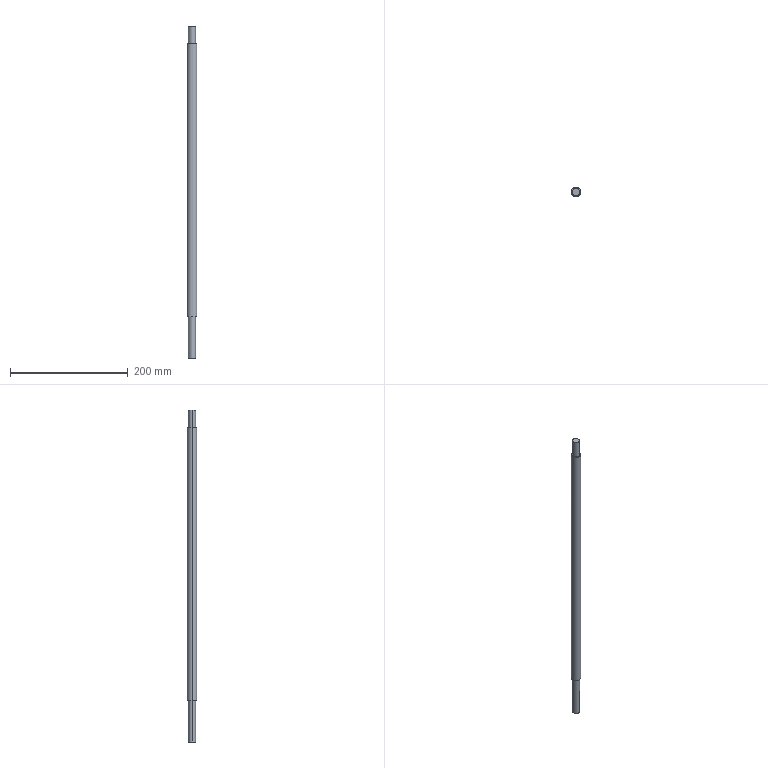Part | SolidWorks | features ICE 2, Extrusion 1 | 1 solid | 10 faces | box 16 x 16 x 563.4 mm | volume 104482 mm3 | cylinder 6 | plane 4 | commonest cylinder face diameters 12 x4 16 x2
STEP:
#1=CARTESIAN_POINT('',(-6.,0.,-301.7));
#2=VERTEX_POINT('',#1);
#3=CARTESIAN_POINT('',(6.,0.,-301.7));
#4=VERTEX_POINT('',#3);
#5=CARTESIAN_POINT('',(0.,0.,-301.7));
#6=DIRECTION('',(0.,0.,-1.));
#7=DIRECTION('',(-1.,0.,0.));
#8=AXIS2_PLACEMENT_3D('',#5,#6,#7);
#9=CIRCLE('',#8,6.);
#10=EDGE_CURVE('',#2,#4,#9,.T.);
#11=ORIENTED_EDGE('',*,*,#10,.F.);
#12=CARTESIAN_POINT('',(-6.,0.,-231.7));
#13=VERTEX_POINT('',#12);
#14=CARTESIAN_POINT('',(-6.,0.,-301.7));
#15=DIRECTION('',(0.,0.,1.));
#16=VECTOR('',#15,1000.);
#17=LINE('',#14,#16);
#18=EDGE_CURVE('',#2,#13,#17,.T.);
#19=ORIENTED_EDGE('',*,*,#18,.T.);
#20=CARTESIAN_POINT('',(6.,0.,-231.7));
#21=VERTEX_POINT('',#20);
#22=CARTESIAN_POINT('',(0.,0.,-231.7));
#23=DIRECTION('',(0.,0.,-1.));
#24=DIRECTION('',(1.,0.,0.));
#25=AXIS2_PLACEMENT_3D('',#22,#23,#24);
#26=CIRCLE('',#25,6.);
#27=EDGE_CURVE('',#13,#21,#26,.T.);
#28=ORIENTED_EDGE('',*,*,#27,.T.);
#29=CARTESIAN_POINT('',(6.,0.,-301.7));
#30=DIRECTION('',(0.,0.,1.));
#31=VECTOR('',#30,1000.);
#32=LINE('',#29,#31);
#33=EDGE_CURVE('',#4,#21,#32,.T.);
#34=ORIENTED_EDGE('',*,*,#33,.F.);
#35=EDGE_LOOP('',(#11,#19,#28,#34));
#36=FACE_OUTER_BOUND('',#35,.T.);
#37=CARTESIAN_POINT('',(0.,0.,-301.7));
#38=DIRECTION('',(0.,0.,1.));
#39=DIRECTION('',(1.,0.,0.));
#40=AXIS2_PLACEMENT_3D('',#37,#38,#39);
#41=CYLINDRICAL_SURFACE('',#40,6.);
#42=ADVANCED_FACE('',(#36),#41,.T.);
#43=CARTESIAN_POINT('',(6.,0.,261.7));
#44=VERTEX_POINT('',#43);
#45=CARTESIAN_POINT('',(-6.,0.,261.7));
#46=VERTEX_POINT('',#45);
#47=CARTESIAN_POINT('',(0.,0.,261.7));
#48=DIRECTION('',(0.,0.,1.));
#49=DIRECTION('',(1.,0.,0.));
#50=AXIS2_PLACEMENT_3D('',#47,#48,#49);
#51=CIRCLE('',#50,6.);
#52=EDGE_CURVE('',#44,#46,#51,.T.);
#53=ORIENTED_EDGE('',*,*,#52,.F.);
#54=CARTESIAN_POINT('',(6.,0.,231.7));
#55=VERTEX_POINT('',#54);
#56=CARTESIAN_POINT('',(6.,0.,261.7));
#57=DIRECTION('',(0.,0.,-1.));
#58=VECTOR('',#57,1000.);
#59=LINE('',#56,#58);
#60=EDGE_CURVE('',#44,#55,#59,.T.);
#61=ORIENTED_EDGE('',*,*,#60,.T.);
#62=CARTESIAN_POINT('',(-6.,0.,231.7));
#63=VERTEX_POINT('',#62);
#64=CARTESIAN_POINT('',(0.,0.,231.7));
#65=DIRECTION('',(0.,0.,1.));
#66=DIRECTION('',(1.,0.,0.));
#67=AXIS2_PLACEMENT_3D('',#64,#65,#66);
#68=CIRCLE('',#67,6.);
#69=EDGE_CURVE('',#55,#63,#68,.T.);
#70=ORIENTED_EDGE('',*,*,#69,.T.);
#71=CARTESIAN_POINT('',(-6.,0.,261.7));
#72=DIRECTION('',(0.,0.,-1.));
#73=VECTOR('',#72,1000.);
#74=LINE('',#71,#73);
#75=EDGE_CURVE('',#46,#63,#74,.T.);
#76=ORIENTED_EDGE('',*,*,#75,.F.);
#77=EDGE_LOOP('',(#53,#61,#70,#76));
#78=FACE_OUTER_BOUND('',#77,.T.);
#79=CARTESIAN_POINT('',(0.,0.,261.7));
#80=DIRECTION('',(0.,0.,-1.));
#81=DIRECTION('',(-1.,0.,0.));
#82=AXIS2_PLACEMENT_3D('',#79,#80,#81);
#83=CYLINDRICAL_SURFACE('',#82,6.);
#84=ADVANCED_FACE('',(#78),#83,.T.);
#85=CARTESIAN_POINT('',(8.,0.,231.7));
#86=VERTEX_POINT('',#85);
#87=CARTESIAN_POINT('',(-8.,0.,231.7));
#88=VERTEX_POINT('',#87);
#89=CARTESIAN_POINT('',(0.,0.,231.7));
#90=DIRECTION('',(0.,0.,1.));
#91=DIRECTION('',(1.,0.,0.));
#92=AXIS2_PLACEMENT_3D('',#89,#90,#91);
#93=CIRCLE('',#92,8.);
#94=EDGE_CURVE('',#86,#88,#93,.T.);
#95=ORIENTED_EDGE('',*,*,#94,.F.);
#96=CARTESIAN_POINT('',(8.,0.,-231.7));
#97=VERTEX_POINT('',#96);
#98=CARTESIAN_POINT('',(8.,0.,231.7));
#99=DIRECTION('',(0.,0.,-1.));
#100=VECTOR('',#99,1000.);
#101=LINE('',#98,#100);
#102=EDGE_CURVE('',#86,#97,#101,.T.);
#103=ORIENTED_EDGE('',*,*,#102,.T.);
#104=CARTESIAN_POINT('',(-8.,0.,-231.7));
#105=VERTEX_POINT('',#104);
#106=CARTESIAN_POINT('',(0.,0.,-231.7));
#107=DIRECTION('',(0.,0.,1.));
#108=DIRECTION('',(1.,0.,0.));
#109=AXIS2_PLACEMENT_3D('',#106,#107,#108);
#110=CIRCLE('',#109,8.);
#111=EDGE_CURVE('',#97,#105,#110,.T.);
#112=ORIENTED_EDGE('',*,*,#111,.T.);
#113=CARTESIAN_POINT('',(-8.,0.,231.7));
#114=DIRECTION('',(0.,0.,-1.));
#115=VECTOR('',#114,1000.);
#116=LINE('',#113,#115);
#117=EDGE_CURVE('',#88,#105,#116,.T.);
#118=ORIENTED_EDGE('',*,*,#117,.F.);
#119=EDGE_LOOP('',(#95,#103,#112,#118));
#120=FACE_OUTER_BOUND('',#119,.T.);
#121=CARTESIAN_POINT('',(0.,0.,231.7));
#122=DIRECTION('',(0.,0.,-1.));
#123=DIRECTION('',(-1.,0.,0.));
#124=AXIS2_PLACEMENT_3D('',#121,#122,#123);
#125=CYLINDRICAL_SURFACE('',#124,8.);
#126=ADVANCED_FACE('',(#120),#125,.T.);
#127=CARTESIAN_POINT('',(0.,0.,-231.7));
#128=DIRECTION('',(0.,0.,1.));
#129=DIRECTION('',(1.,0.,0.));
#130=AXIS2_PLACEMENT_3D('',#127,#128,#129);
#131=CIRCLE('',#130,8.);
#132=EDGE_CURVE('',#105,#97,#131,.T.);
#133=ORIENTED_EDGE('',*,*,#132,.F.);
#134=ORIENTED_EDGE('',*,*,#111,.F.);
#135=EDGE_LOOP('',(#133,#134));
#136=FACE_OUTER_BOUND('',#135,.T.);
#137=CARTESIAN_POINT('',(0.,0.,-231.7));
#138=DIRECTION('',(0.,0.,-1.));
#139=DIRECTION('',(1.,0.,0.));
#140=AXIS2_PLACEMENT_3D('',#137,#138,#139);
#141=CIRCLE('',#140,6.);
#142=EDGE_CURVE('',#21,#13,#141,.T.);
#143=ORIENTED_EDGE('',*,*,#142,.F.);
#144=ORIENTED_EDGE('',*,*,#27,.F.);
#145=EDGE_LOOP('',(#143,#144));
#146=FACE_BOUND('',#145,.T.);
#147=CARTESIAN_POINT('',(0.,0.,-231.7));
#148=DIRECTION('',(0.,0.,1.));
#149=DIRECTION('',(1.,0.,0.));
#150=AXIS2_PLACEMENT_3D('',#147,#148,#149);
#151=PLANE('',#150);
#152=ADVANCED_FACE('',(#136,#146),#151,.F.);
#153=CARTESIAN_POINT('',(0.,0.,231.7));
#154=DIRECTION('',(0.,0.,1.));
#155=DIRECTION('',(1.,0.,0.));
#156=AXIS2_PLACEMENT_3D('',#153,#154,#155);
#157=CIRCLE('',#156,8.);
#158=EDGE_CURVE('',#88,#86,#157,.T.);
#159=ORIENTED_EDGE('',*,*,#158,.T.);
#160=ORIENTED_EDGE('',*,*,#94,.T.);
#161=EDGE_LOOP('',(#159,#160));
#162=FACE_OUTER_BOUND('',#161,.T.);
#163=CARTESIAN_POINT('',(0.,0.,231.7));
#164=DIRECTION('',(0.,0.,1.));
#165=DIRECTION('',(1.,0.,0.));
#166=AXIS2_PLACEMENT_3D('',#163,#164,#165);
#167=CIRCLE('',#166,6.);
#168=EDGE_CURVE('',#63,#55,#167,.T.);
#169=ORIENTED_EDGE('',*,*,#168,.F.);
#170=ORIENTED_EDGE('',*,*,#69,.F.);
#171=EDGE_LOOP('',(#169,#170));
#172=FACE_BOUND('',#171,.T.);
#173=CARTESIAN_POINT('',(0.,0.,231.7));
#174=DIRECTION('',(0.,0.,1.));
#175=DIRECTION('',(1.,0.,0.));
#176=AXIS2_PLACEMENT_3D('',#173,#174,#175);
#177=PLANE('',#176);
#178=ADVANCED_FACE('',(#162,#172),#177,.T.);
#179=ORIENTED_EDGE('',*,*,#102,.F.);
#180=ORIENTED_EDGE('',*,*,#158,.F.);
#181=ORIENTED_EDGE('',*,*,#117,.T.);
#182=ORIENTED_EDGE('',*,*,#132,.T.);
#183=EDGE_LOOP('',(#179,#180,#181,#182));
#184=FACE_OUTER_BOUND('',#183,.T.);
#185=CARTESIAN_POINT('',(0.,0.,231.7));
#186=DIRECTION('',(0.,0.,-1.));
#187=DIRECTION('',(-1.,0.,0.));
#188=AXIS2_PLACEMENT_3D('',#185,#186,#187);
#189=CYLINDRICAL_SURFACE('',#188,8.);
#190=ADVANCED_FACE('',(#184),#189,.T.);
#191=ORIENTED_EDGE('',*,*,#60,.F.);
#192=CARTESIAN_POINT('',(0.,0.,261.7));
#193=DIRECTION('',(0.,0.,1.));
#194=DIRECTION('',(1.,0.,0.));
#195=AXIS2_PLACEMENT_3D('',#192,#193,#194);
#196=CIRCLE('',#195,6.);
#197=EDGE_CURVE('',#46,#44,#196,.T.);
#198=ORIENTED_EDGE('',*,*,#197,.F.);
#199=ORIENTED_EDGE('',*,*,#75,.T.);
#200=ORIENTED_EDGE('',*,*,#168,.T.);
#201=EDGE_LOOP('',(#191,#198,#199,#200));
#202=FACE_OUTER_BOUND('',#201,.T.);
#203=CARTESIAN_POINT('',(0.,0.,261.7));
#204=DIRECTION('',(0.,0.,-1.));
#205=DIRECTION('',(-1.,0.,0.));
#206=AXIS2_PLACEMENT_3D('',#203,#204,#205);
#207=CYLINDRICAL_SURFACE('',#206,6.);
#208=ADVANCED_FACE('',(#202),#207,.T.);
#209=ORIENTED_EDGE('',*,*,#197,.T.);
#210=ORIENTED_EDGE('',*,*,#52,.T.);
#211=EDGE_LOOP('',(#209,#210));
#212=FACE_OUTER_BOUND('',#211,.T.);
#213=CARTESIAN_POINT('',(0.,0.,261.7));
#214=DIRECTION('',(0.,0.,1.));
#215=DIRECTION('',(1.,0.,0.));
#216=AXIS2_PLACEMENT_3D('',#213,#214,#215);
#217=PLANE('',#216);
#218=ADVANCED_FACE('',(#212),#217,.T.);
#219=ORIENTED_EDGE('',*,*,#18,.F.);
#220=CARTESIAN_POINT('',(0.,0.,-301.7));
#221=DIRECTION('',(0.,0.,-1.));
#222=DIRECTION('',(-1.,0.,0.));
#223=AXIS2_PLACEMENT_3D('',#220,#221,#222);
#224=CIRCLE('',#223,6.);
#225=EDGE_CURVE('',#4,#2,#224,.T.);
#226=ORIENTED_EDGE('',*,*,#225,.F.);
#227=ORIENTED_EDGE('',*,*,#33,.T.);
#228=ORIENTED_EDGE('',*,*,#142,.T.);
#229=EDGE_LOOP('',(#219,#226,#227,#228));
#230=FACE_OUTER_BOUND('',#229,.T.);
#231=CARTESIAN_POINT('',(0.,0.,-301.7));
#232=DIRECTION('',(0.,0.,1.));
#233=DIRECTION('',(1.,0.,0.));
#234=AXIS2_PLACEMENT_3D('',#231,#232,#233);
#235=CYLINDRICAL_SURFACE('',#234,6.);
#236=ADVANCED_FACE('',(#230),#235,.T.);
#237=ORIENTED_EDGE('',*,*,#225,.T.);
#238=ORIENTED_EDGE('',*,*,#10,.T.);
#239=EDGE_LOOP('',(#237,#238));
#240=FACE_OUTER_BOUND('',#239,.T.);
#241=CARTESIAN_POINT('',(0.,0.,-301.7));
#242=DIRECTION('',(0.,0.,-1.));
#243=DIRECTION('',(-1.,0.,0.));
#244=AXIS2_PLACEMENT_3D('',#241,#242,#243);
#245=PLANE('',#244);
#246=ADVANCED_FACE('',(#240),#245,.T.);
#247=CLOSED_SHELL('',(#42,#84,#126,#152,#178,#190,#208,#218,#236,#246));
#248=MANIFOLD_SOLID_BREP('',#247);
#249=CARTESIAN_POINT('',(0.,0.,0.));
#250=DIRECTION('',(0.,0.,1.));
#251=DIRECTION('',(1.,0.,0.));
#252=AXIS2_PLACEMENT_3D('',#249,#250,#251);
#253=(LENGTH_UNIT()NAMED_UNIT(*)SI_UNIT(.MILLI.,.METRE.));
#254=UNCERTAINTY_MEASURE_WITH_UNIT(LENGTH_MEASURE(0.00001),#253,'','');
#255=(NAMED_UNIT(*)PLANE_ANGLE_UNIT()SI_UNIT($,.RADIAN.));
#256=(NAMED_UNIT(*)SI_UNIT($,.STERADIAN.)SOLID_ANGLE_UNIT());
#257=(GEOMETRIC_REPRESENTATION_CONTEXT(3)GLOBAL_UNCERTAINTY_ASSIGNED_CONTEXT((#254))GLOBAL_UNIT_ASSIGNED_CONTEXT((#253,#255,#256))REPRESENTATION_CONTEXT('',''));
#258=ADVANCED_BREP_SHAPE_REPRESENTATION('',(#248,#252),#257);